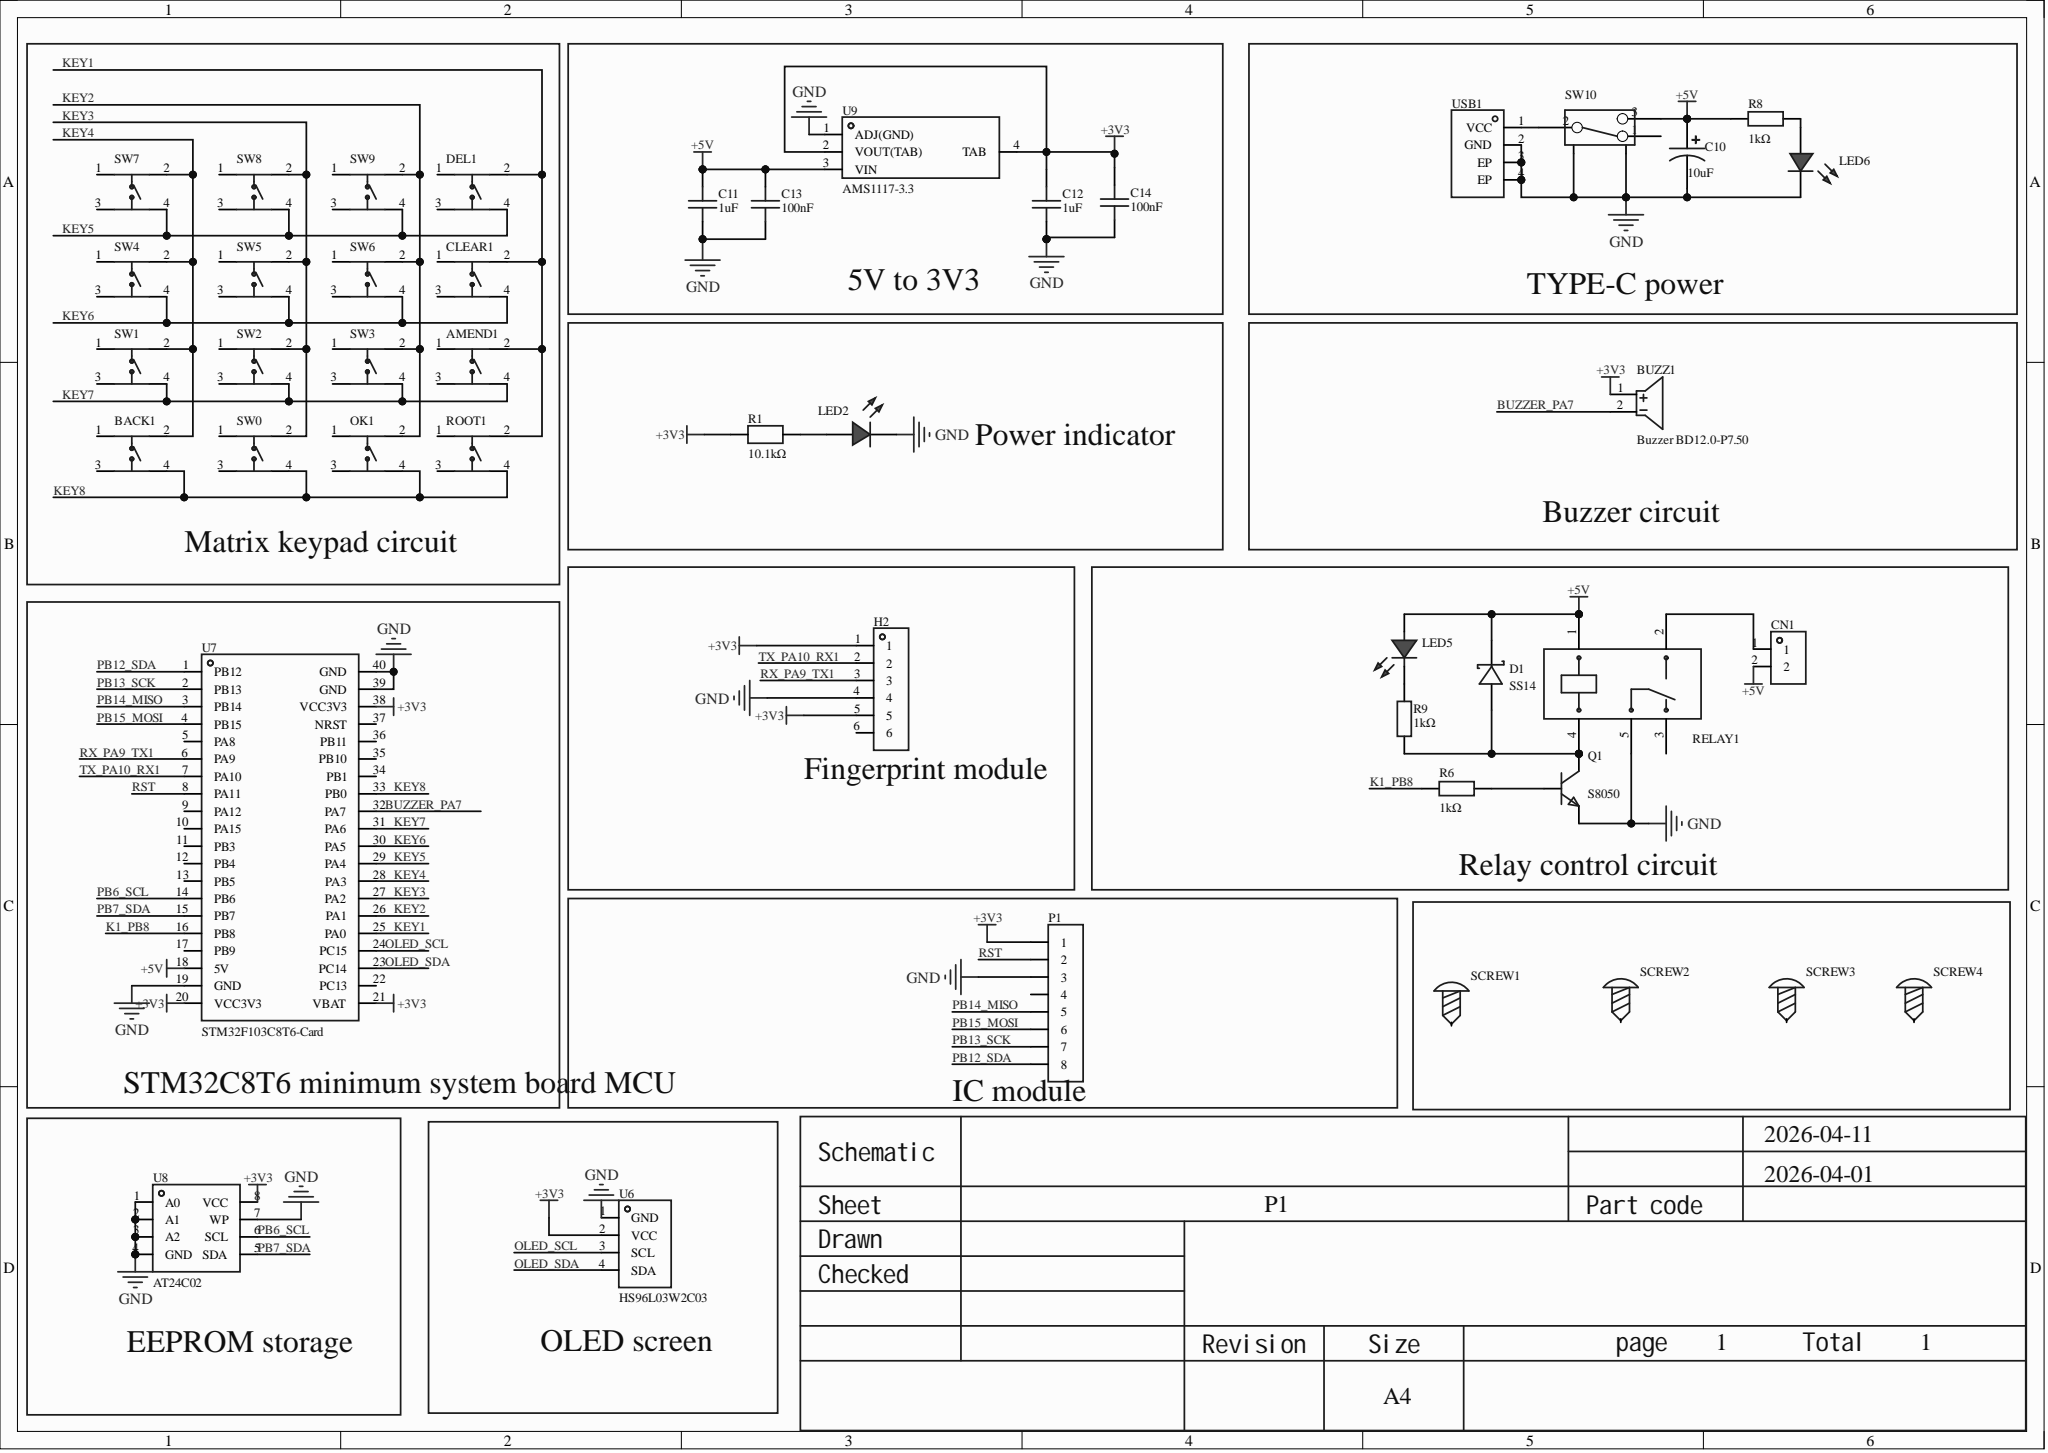Circuit board | Altium Designer | 45 parts | 31 nets
Bill of materials:
Comment,Description,Designator,Footprint,LibRef,Quantity
"KH-6X6X5H-STM","","AMEND1, BACK1, CLEAR1, DEL1, OK1, ROOT1, SW0, SW1, SW2, SW3, SW4, SW5, SW6, SW7, SW8, SW9","SW-SMD_4P-L6.0-W6.0-P4.50-LS9.0-2","KH-6X6X5H-STM","16"
"Buzzer BD12.0-P7.50","","BUZZ1","BUZ-TH_BD12.0-P7.50-D0.6-FD","蜂鸣器BD12.0-P7.50","1"
"10uF","Capacitance: 10uF; tolerance: ±20%; rated voltage: 50V; ripple current: 50mA@120Hz; ESR: -;","C10","CAP-TH_BD5.0-P2.00-D0.8-FD","01EC1809SHC10UF50V","1"
"1uF","Capacitance: 1uF; tolerance: ±10%; rated voltage: 50V; dielectric (temperature coefficient): X5R;","C11, C12","C0603","CL10A105KB8NNNC","2"
"100nF","Capacitance: 100nF; tolerance: ±10%; rated voltage: 50V; dielectric (temperature coefficient): X7R;","C13, C14","C0603","CC0603KRX7R9BB104","2"
"ZX-XH2.54-2PZZ","","CN1","CONN-TH_2P-P2.50_HX25003-2A","ZX-XH2.54-2PZZ","1"
"SS14","Diode configuration: independent; forward voltage (Vf): 550mV@1A; DC reverse voltage (Vr): 40V; rectifier current: 1A;","D1","SMA_L4.2-W2.6-LS5.3-RD","SS14_C2480","1"
"PM254V-11-06-H85","","H2","hdr-th_6p-p2.54-v-f","PM254V-11-06-H85","1"
"","","LED2, LED6","LED-TH_5mm","LED_TH-R_5mm","2"
"XL-302SURD","","LED5","LED-TH_BD3.8-P2.54-RD","XL-302SURD","1"
"2.54-1*8P female, RoHS","Socket structure: 1x8P; pitch: 2.54mm; row spacing: -; mounting type: through-hole; rows: single row; total positions: 8P; plastic height: -; contact material: -; contact plating: -;","P1","HDR-TH_8P-P2.54-V-F-1","2.54-1*8P母环保","1"
"S8050","Transistor type: NPN; collector current (Ic): 500mA; collector-emitter breakdown voltage (Vceo): 25V; power (Pd): 300mW;","Q1","SOT-23-3_L2.9-W1.6-P1.90-LS2.8-BR","S8050_C181158","1"
"10.1kΩ","Resistor type: thin film; resistance: 10.1kΩ; tolerance: ±0.1%; power: 125mW; temperature coefficient: ±25ppm/?;","R1","R0805","RT0805BRD0710K1L","1"
"1kΩ","Resistor type: thick film; resistance: 1kΩ; tolerance: ±1%; power: 100mW; max working voltage: 75V; temperature coefficient: ±100ppm/?;","R6","R0603","RC0603FR-071KL","1"
"1kΩ","Resistor type: metal film; resistance: 1kΩ; tolerance: ±1%; power: 250mW; temperature coefficient: ±50ppm/?;","R8, R9","RES-TH_BD2.5-L6.5-P10.50-D0.6","MFR0W4F1001A50","2"
"SRD-12VDC-SL-C","Coil voltage: 12V; contact form: changeover 1C (SPDT); contact rating (resistive load): -; max switching voltage: 250V@AC; max switching current: 15A;","RELAY1","RELAY-TH_SRD-XXVDC-XL-C","SRD-12VDC-SL-C","1"
"","","SCREW1, SCREW2, SCREW3, SCREW4","M3螺丝","M3螺丝","4"
"SK-12E12-G5","Circuit structure: SPDT; mounting style: side entry; rated current (DC): -; rated voltage (DC): -; rated current (AC): -; rated voltage (AC): -; mechanical life: 5 thousand cycles;","SW10","SW-TH_SK-12E12-G5","SK-12E12-G5","1"
"HS96L03W2C03","Main controller chip: SSD1315; interface type: I2C; size (inch): 0.96; pixel resolution: 128x64;","U6","OLED-TH_L27.8-W27.2-P2.54_C9900033791","HS96L03W2C03","1"
"STM32F103C8T6-Card","","U7","CONN-TH_L53.3-W22.9_STM32F103C8T6-CARD","STM32F103C8T6-Card","1"
"AT24C02","","U8","SOP-8_L5.0-W4.0-P1.27-LS6.0-BL","AT24C02_C688857","1"
"AMS1117-3.3","Output type: fixed; max input voltage: 12V; output voltage: 3.3V; max output current: 1A; PSRR: 60dB@(120Hz); output polarity: positive;","U9","SOT-223-4_L6.5-W3.5-P2.30-LS7.0-BR","AMS1117-3.3_C347222","1"
"KH-TYPE-C-2P","Connector type: Type-C; standard: -; male/female: -; port count: -; contact count: 2P; mounting: -; rated current - power: -; contact material: -; contact plating: -; operating temperature range: -;","USB1","USB-SMD_KH-TYPE-C-2P","KH-TYPE-C-2P","1"
Netlist (Protel format):
[
AMEND1
SW-SMD_4P-L6.0-W6.0-P4.50-LS9.0-2
KH-6X6X5H-STM



]
[
BACK1
SW-SMD_4P-L6.0-W6.0-P4.50-LS9.0-2
KH-6X6X5H-STM



]
[
BUZZ1
BUZ-TH_BD12.0-P7.50-D0.6-FD
Buzzer BD12.0-P7.50



]
[
C10
CAP-TH_BD5.0-P2.00-D0.8-FD
10uF



]
[
C11
C0603
1uF



]
[
C12
C0603
1uF



]
[
C13
C0603
100nF



]
[
C14
C0603
100nF



]
[
CLEAR1
SW-SMD_4P-L6.0-W6.0-P4.50-LS9.0-2
KH-6X6X5H-STM



]
[
CN1
CONN-TH_2P-P2.50_HX25003-2A
ZX-XH2.54-2PZZ



]
[
D1
SMA_L4.2-W2.6-LS5.3-RD
SS14



]
[
DEL1
SW-SMD_4P-L6.0-W6.0-P4.50-LS9.0-2
KH-6X6X5H-STM



]
[
H2
hdr-th_6p-p2.54-v-f
PM254V-11-06-H85



]
[
LED2
LED-TH_5mm




]
[
LED5
LED-TH_BD3.8-P2.54-RD
XL-302SURD



]
[
LED6
LED-TH_5mm




]
[
OK1
SW-SMD_4P-L6.0-W6.0-P4.50-LS9.0-2
KH-6X6X5H-STM



]
[
P1
HDR-TH_8P-P2.54-V-F-1
2.54-1*8P female, RoHS



]
[
Q1
SOT-23-3_L2.9-W1.6-P1.90-LS2.8-BR
S8050



]
[
R1
R0805
10.1kΩ



]
[
R6
R0603
1kΩ



]
[
R8
RES-TH_BD2.5-L6.5-P10.50-D0.6
1kΩ



]
[
R9
RES-TH_BD2.5-L6.5-P10.50-D0.6
1kΩ



]
[
RELAY1
RELAY-TH_SRD-XXVDC-XL-C
SRD-12VDC-SL-C



]
[
ROOT1
SW-SMD_4P-L6.0-W6.0-P4.50-LS9.0-2
KH-6X6X5H-STM



]
[
SCREW1
M3螺丝




]
[
SCREW2
M3螺丝




]
[
SCREW3
M3螺丝




]
[
SCREW4
M3螺丝




]
[
SW0
SW-SMD_4P-L6.0-W6.0-P4.50-LS9.0-2
KH-6X6X5H-STM



]
[
SW1
SW-SMD_4P-L6.0-W6.0-P4.50-LS9.0-2
KH-6X6X5H-STM



]
[
SW2
SW-SMD_4P-L6.0-W6.0-P4.50-LS9.0-2
KH-6X6X5H-STM



]
[
SW3
SW-SMD_4P-L6.0-W6.0-P4.50-LS9.0-2
KH-6X6X5H-STM



]
[
SW4
SW-SMD_4P-L6.0-W6.0-P4.50-LS9.0-2
KH-6X6X5H-STM



]
[
SW5
SW-SMD_4P-L6.0-W6.0-P4.50-LS9.0-2
KH-6X6X5H-STM



]
[
SW6
SW-SMD_4P-L6.0-W6.0-P4.50-LS9.0-2
KH-6X6X5H-STM



]
[
SW7
SW-SMD_4P-L6.0-W6.0-P4.50-LS9.0-2
KH-6X6X5H-STM



]
[
SW8
SW-SMD_4P-L6.0-W6.0-P4.50-LS9.0-2
KH-6X6X5H-STM



]
[
SW9
SW-SMD_4P-L6.0-W6.0-P4.50-LS9.0-2
KH-6X6X5H-STM



]
[
SW10
SW-TH_SK-12E12-G5
SK-12E12-G5



]
[
U6
OLED-TH_L27.8-W27.2-P2.54_C9900033791
HS96L03W2C03



]
[
U7
CONN-TH_L53.3-W22.9_STM32F103C8T6-CARD
STM32F103C8T6-Card



]
[
U8
SOP-8_L5.0-W4.0-P1.27-LS6.0-BL
AT24C02



]
[
U9
SOT-223-4_L6.5-W3.5-P2.30-LS7.0-BR
AMS1117-3.3



]
[
USB1
USB-SMD_KH-TYPE-C-2P
KH-TYPE-C-2P



]
(
TX_PA10_RX1
H2-2
U7-7
)
(
RX_PA9_TX1
H2-3
U7-6
)
(
RST
P1-2
U7-8
)
(
PB15_MOSI
P1-6
U7-4
)
(
PB14_MISO
P1-5
U7-3
)
(
PB13_SCK
P1-7
U7-2
)
(
PB12_SDA
P1-8
U7-1
)
(
PB7_SDA
U7-15
U8-5
)
(
PB6_SCL
U7-14
U8-6
)
(
OLED_SDA
U6-4
U7-23
)
(
OLED_SCL
U6-3
U7-24
)
(
NetSW10_2
SW10-2
USB1-1
)
(
NetQ1_1
Q1-1
R6-1
)
(
NetLED6_1
LED6-1
R8-2
)
(
NetLED5_1
LED5-1
R9-2
)
(
NetLED2_1
LED2-1
R1-2
)
(
NetD1_2
D1-2
Q1-3
R9-1
RELAY1-4
)
(
NetCN1_1
CN1-1
RELAY1-2
)
(
KEY8
BACK1-4
OK1-4
ROOT1-4
SW0-4
U7-33
)
(
KEY7
AMEND1-4
SW1-4
SW2-4
SW3-4
U7-31
)
(
KEY6
CLEAR1-4
SW4-4
SW5-4
SW6-4
U7-30
)
(
KEY5
DEL1-4
SW7-4
SW8-4
SW9-4
U7-29
)
(
KEY4
BACK1-2
SW1-2
SW4-2
SW7-2
U7-28
)
(
KEY3
SW0-2
SW2-2
SW5-2
SW8-2
U7-27
)
(
KEY2
OK1-2
SW3-2
SW6-2
SW9-2
U7-26
)
(
KEY1
AMEND1-2
CLEAR1-2
DEL1-2
ROOT1-2
U7-25
)
(
K1_PB8
R6-2
U7-16
)
(
GND
C10-2
C11-1
C12-1
C13-1
C14-1
H2-4
LED2-2
LED6-2
P1-3
Q1-2
RELAY1-5
SW10-4
SW10-5
U6-1
U7-19
U7-39
U7-40
U8-1
U8-2
U8-3
U8-4
U8-7
U9-1
USB1-2
USB1-3
USB1-4
)
(
BUZZER_PA7
BUZZ1-2
U7-32
)
(
+5V
C10-1
C11-2
C13-2
CN1-2
D1-1
LED5-2
R8-1
RELAY1-1
SW10-3
U7-18
U9-3
)
(
+3V3
BUZZ1-1
C12-2
C14-2
H2-1
H2-5
P1-1
R1-1
U6-2
U7-20
U7-21
U7-38
U8-8
U9-2
U9-4
)